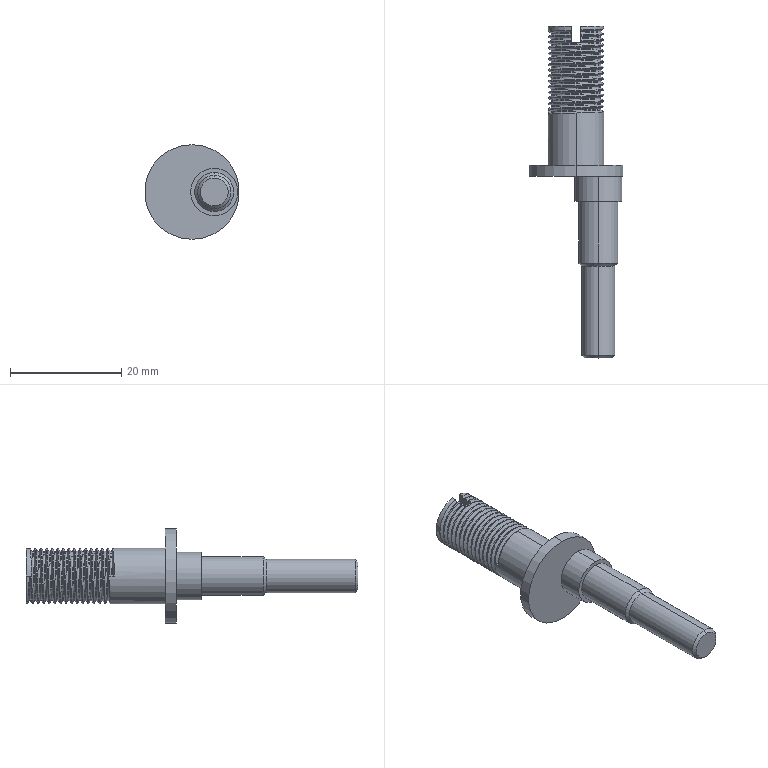Part | SolidWorks | features ICE 5, Chamfer 2, Extrusion 1, SweepThread 1 | 1 solid | 72 faces | box 17 x 59.6 x 17 mm | volume 3396 mm3 | cylinder 40 | spline 17 | plane 11 | cone 4 | commonest cylinder face diameters 10 x32 6 x2 7 x2 8.5 x2 17 x2